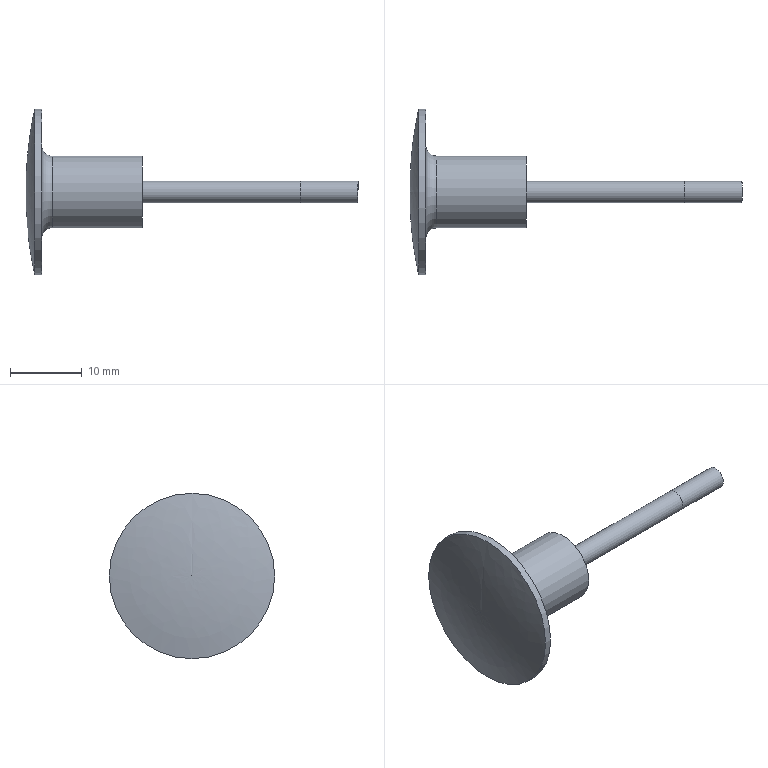Part | STEP file | 1-29.2 | 1 solid | 9 faces | box 46.201 x 23 x 23 mm | volume 2003 mm3 | cylinder 4 | plane 3 | spline 1 | torus 1 | commonest cylinder face diameters 3 x2 10 x1 23 x1
STEP:
#1=CARTESIAN_POINT('',(0.,0.,0.));
#2=DIRECTION('',(0.,0.,1.));
#3=DIRECTION('',(1.,0.,0.));
#4=AXIS2_PLACEMENT_3D('',#1,#2,#3);
#5=CARTESIAN_POINT('',(0.,11.5,0.));
#6=VERTEX_POINT('',#5);
#7=CARTESIAN_POINT('',(-1.,11.5,0.));
#8=VERTEX_POINT('',#7);
#9=CARTESIAN_POINT('',(0.,11.5,0.));
#10=DIRECTION('',(-1.,0.,0.));
#11=VECTOR('',#10,1.);
#12=LINE('',#9,#11);
#13=CARTESIAN_POINT('',(0.,0.,0.));
#14=DIRECTION('',(-1.,0.,0.));
#15=DIRECTION('',(0.,1.,0.));
#16=AXIS2_PLACEMENT_3D('',#13,#14,#15);
#17=CYLINDRICAL_SURFACE('',#16,11.5);
#18=CARTESIAN_POINT('',(6.283,0.));
#19=DIRECTION('',(0.,1.));
#20=VECTOR('',#19,1.);
#21=LINE('',#18,#20);
#22=(GEOMETRIC_REPRESENTATION_CONTEXT(2)PARAMETRIC_REPRESENTATION_CONTEXT()REPRESENTATION_CONTEXT('',''));
#23=DEFINITIONAL_REPRESENTATION('',(#21),#22);
#24=PCURVE('',#17,#23);
#25=CARTESIAN_POINT('',(0.,0.));
#26=DIRECTION('',(0.,1.));
#27=VECTOR('',#26,1.);
#28=LINE('',#25,#27);
#29=(GEOMETRIC_REPRESENTATION_CONTEXT(2)PARAMETRIC_REPRESENTATION_CONTEXT()REPRESENTATION_CONTEXT('',''));
#30=DEFINITIONAL_REPRESENTATION('',(#28),#29);
#31=PCURVE('',#17,#30);
#32=SEAM_CURVE('',#12,(#24,#31),.PCURVE_S1.);
#33=EDGE_CURVE('',#6,#8,#32,.T.);
#34=ORIENTED_EDGE('',*,*,#33,.T.);
#35=CARTESIAN_POINT('',(-1.,0.,11.5));
#36=VERTEX_POINT('',#35);
#37=CARTESIAN_POINT('',(-1.,0.,0.));
#38=DIRECTION('',(1.,0.,0.));
#39=DIRECTION('',(0.,1.,0.));
#40=AXIS2_PLACEMENT_3D('',#37,#38,#39);
#41=CIRCLE('',#40,11.5);
#42=CARTESIAN_POINT('',(6.283,1.));
#43=DIRECTION('',(-1.,0.));
#44=VECTOR('',#43,1.);
#45=LINE('',#42,#44);
#46=(GEOMETRIC_REPRESENTATION_CONTEXT(2)PARAMETRIC_REPRESENTATION_CONTEXT()REPRESENTATION_CONTEXT('',''));
#47=DEFINITIONAL_REPRESENTATION('',(#45),#46);
#48=PCURVE('',#17,#47);
#49=CARTESIAN_POINT('',(-1.,0.,11.5));
#50=CARTESIAN_POINT('',(-1.,-11.5,11.5));
#51=CARTESIAN_POINT('',(-1.,-11.5,0.));
#52=CARTESIAN_POINT('',(-1.,-11.5,-11.5));
#53=CARTESIAN_POINT('',(-1.,0.,-11.5));
#54=CARTESIAN_POINT('',(-1.,11.5,-11.5));
#55=CARTESIAN_POINT('',(-1.,11.5,0.));
#56=CARTESIAN_POINT('',(-1.,11.5,11.5));
#57=CARTESIAN_POINT('',(-1.,0.,11.5));
#58=CARTESIAN_POINT('',(-2.243,0.,5.817));
#59=CARTESIAN_POINT('',(-2.243,-5.817,5.817));
#60=CARTESIAN_POINT('',(-2.243,-5.817,0.));
#61=CARTESIAN_POINT('',(-2.243,-5.817,-5.817));
#62=CARTESIAN_POINT('',(-2.243,0.,-5.817));
#63=CARTESIAN_POINT('',(-2.243,5.817,-5.817));
#64=CARTESIAN_POINT('',(-2.243,5.817,0.));
#65=CARTESIAN_POINT('',(-2.243,5.817,5.817));
#66=CARTESIAN_POINT('',(-2.243,0.,5.817));
#67=CARTESIAN_POINT('',(-2.2,0.,0.));
#68=CARTESIAN_POINT('',(-2.2,0.,0.));
#69=CARTESIAN_POINT('',(-2.2,0.,0.));
#70=CARTESIAN_POINT('',(-2.2,0.,0.));
#71=CARTESIAN_POINT('',(-2.2,0.,0.));
#72=CARTESIAN_POINT('',(-2.2,0.,0.));
#73=CARTESIAN_POINT('',(-2.2,0.,0.));
#74=CARTESIAN_POINT('',(-2.2,0.,0.));
#75=CARTESIAN_POINT('',(-2.2,0.,0.));
#76=(BOUNDED_SURFACE()B_SPLINE_SURFACE(2,2,((#49,#50,#51,#52,#53,#54,#55,#56,#57),(#58,#59,#60,#61,#62,#63,#64,#65,#66),(#67,#68,#69,#70,#71,#72,#73,#74,#75)),.UNSPECIFIED.,.F.,.T.,.F.)B_SPLINE_SURFACE_WITH_KNOTS((3,3),(1,2,2,2,2,2,1),(0.,1.),(-0.25,0.,0.25,0.5,0.75,1.,1.25),.UNSPECIFIED.)GEOMETRIC_REPRESENTATION_ITEM()RATIONAL_B_SPLINE_SURFACE(((1.,0.7071,1.,0.7071,1.,0.7071,1.,0.7071,1.),(0.9938,0.7027,0.9938,0.7027,0.9938,0.7027,0.9938,0.7027,0.9938),(1.,0.7071,1.,0.7071,1.,0.7071,1.,0.7071,1.)))REPRESENTATION_ITEM('')SURFACE());
#77=CARTESIAN_POINT('',(0.,0.75));
#78=CARTESIAN_POINT('',(0.,0.7542));
#79=CARTESIAN_POINT('',(0.,0.7625));
#80=CARTESIAN_POINT('',(0.,0.7746));
#81=CARTESIAN_POINT('',(0.,0.7864));
#82=CARTESIAN_POINT('',(0.,0.798));
#83=CARTESIAN_POINT('',(0.,0.8094));
#84=CARTESIAN_POINT('',(0.,0.8206));
#85=CARTESIAN_POINT('',(0.,0.8316));
#86=CARTESIAN_POINT('',(0.,0.8426));
#87=CARTESIAN_POINT('',(0.,0.8534));
#88=CARTESIAN_POINT('',(0.,0.8642));
#89=CARTESIAN_POINT('',(0.,0.875));
#90=CARTESIAN_POINT('',(0.,0.8858));
#91=CARTESIAN_POINT('',(0.,0.8966));
#92=CARTESIAN_POINT('',(0.,0.9074));
#93=CARTESIAN_POINT('',(0.,0.9184));
#94=CARTESIAN_POINT('',(0.,0.9294));
#95=CARTESIAN_POINT('',(0.,0.9406));
#96=CARTESIAN_POINT('',(0.,0.952));
#97=CARTESIAN_POINT('',(0.,0.9636));
#98=CARTESIAN_POINT('',(0.,0.9754));
#99=CARTESIAN_POINT('',(0.,0.9875));
#100=CARTESIAN_POINT('',(0.,0.9958));
#101=CARTESIAN_POINT('',(0.,1.));
#102=B_SPLINE_CURVE_WITH_KNOTS('',3,(#77,#78,#79,#80,#81,#82,#83,#84,#85,#86,#87,#88,#89,#90,#91,#92,#93,#94,#95,#96,#97,#98,#99,#100,#101),.UNSPECIFIED.,.F.,.F.,(4,1,1,1,1,1,1,1,1,1,1,1,1,1,1,1,1,1,1,1,1,1,4),(0.,0.0714,0.1428,0.2142,0.2856,0.357,0.4284,0.4998,0.5712,0.6426,0.714,0.7854,0.8568,0.9282,0.9996,1.071,1.142,1.214,1.285,1.357,1.428,1.499,1.571),.QUASI_UNIFORM_KNOTS.);
#103=(GEOMETRIC_REPRESENTATION_CONTEXT(2)PARAMETRIC_REPRESENTATION_CONTEXT()REPRESENTATION_CONTEXT('',''));
#104=DEFINITIONAL_REPRESENTATION('',(#102),#103);
#105=PCURVE('',#76,#104);
#106=SURFACE_CURVE('',#41,(#48,#105),.PCURVE_S1.);
#107=EDGE_CURVE('',#8,#36,#106,.T.);
#108=ORIENTED_EDGE('',*,*,#107,.T.);
#109=CARTESIAN_POINT('',(-1.,0.,0.));
#110=DIRECTION('',(1.,0.,0.));
#111=DIRECTION('',(0.,0.,1.));
#112=AXIS2_PLACEMENT_3D('',#109,#110,#111);
#113=CIRCLE('',#112,11.5);
#114=CARTESIAN_POINT('',(4.712,1.));
#115=DIRECTION('',(-1.,0.));
#116=VECTOR('',#115,1.);
#117=LINE('',#114,#116);
#118=(GEOMETRIC_REPRESENTATION_CONTEXT(2)PARAMETRIC_REPRESENTATION_CONTEXT()REPRESENTATION_CONTEXT('',''));
#119=DEFINITIONAL_REPRESENTATION('',(#117),#118);
#120=PCURVE('',#17,#119);
#121=CARTESIAN_POINT('',(0.,0.));
#122=CARTESIAN_POINT('',(0.,0.0126));
#123=CARTESIAN_POINT('',(0.,0.03676));
#124=CARTESIAN_POINT('',(0.,0.07076));
#125=CARTESIAN_POINT('',(0.,0.1035));
#126=CARTESIAN_POINT('',(0.,0.1357));
#127=CARTESIAN_POINT('',(0.,0.1682));
#128=CARTESIAN_POINT('',(0.,0.2017));
#129=CARTESIAN_POINT('',(0.,0.2371));
#130=CARTESIAN_POINT('',(0.,0.2752));
#131=CARTESIAN_POINT('',(0.,0.3096));
#132=CARTESIAN_POINT('',(0.,0.3427));
#133=CARTESIAN_POINT('',(0.,0.375));
#134=CARTESIAN_POINT('',(0.,0.4073));
#135=CARTESIAN_POINT('',(0.,0.4404));
#136=CARTESIAN_POINT('',(0.,0.4748));
#137=CARTESIAN_POINT('',(0.,0.5129));
#138=CARTESIAN_POINT('',(0.,0.5483));
#139=CARTESIAN_POINT('',(0.,0.5818));
#140=CARTESIAN_POINT('',(0.,0.6143));
#141=CARTESIAN_POINT('',(0.,0.6465));
#142=CARTESIAN_POINT('',(0.,0.6792));
#143=CARTESIAN_POINT('',(0.,0.7132));
#144=CARTESIAN_POINT('',(0.,0.7374));
#145=CARTESIAN_POINT('',(0.,0.75));
#146=B_SPLINE_CURVE_WITH_KNOTS('',3,(#121,#122,#123,#124,#125,#126,#127,#128,#129,#130,#131,#132,#133,#134,#135,#136,#137,#138,#139,#140,#141,#142,#143,#144,#145),.UNSPECIFIED.,.F.,.F.,(4,1,1,1,1,1,1,1,1,1,1,1,1,1,1,1,1,1,1,1,1,1,4),(0.,0.2142,0.4284,0.6426,0.8568,1.071,1.285,1.499,1.714,1.928,2.142,2.356,2.57,2.785,2.999,3.213,3.427,3.641,3.856,4.07,4.284,4.498,4.712),.QUASI_UNIFORM_KNOTS.);
#147=(GEOMETRIC_REPRESENTATION_CONTEXT(2)PARAMETRIC_REPRESENTATION_CONTEXT()REPRESENTATION_CONTEXT('',''));
#148=DEFINITIONAL_REPRESENTATION('',(#146),#147);
#149=PCURVE('',#76,#148);
#150=SURFACE_CURVE('',#113,(#120,#149),.PCURVE_S1.);
#151=EDGE_CURVE('',#36,#8,#150,.T.);
#152=ORIENTED_EDGE('',*,*,#151,.T.);
#153=ORIENTED_EDGE('',*,*,#33,.F.);
#154=CARTESIAN_POINT('',(0.,0.,0.));
#155=DIRECTION('',(1.,0.,0.));
#156=DIRECTION('',(0.,1.,0.));
#157=AXIS2_PLACEMENT_3D('',#154,#155,#156);
#158=CIRCLE('',#157,11.5);
#159=CARTESIAN_POINT('',(6.283,0.));
#160=DIRECTION('',(-1.,0.));
#161=VECTOR('',#160,1.);
#162=LINE('',#159,#161);
#163=(GEOMETRIC_REPRESENTATION_CONTEXT(2)PARAMETRIC_REPRESENTATION_CONTEXT()REPRESENTATION_CONTEXT('',''));
#164=DEFINITIONAL_REPRESENTATION('',(#162),#163);
#165=PCURVE('',#17,#164);
#166=CARTESIAN_POINT('',(0.,-3.081,0.));
#167=DIRECTION('',(1.,0.,0.));
#168=DIRECTION('',(0.,0.,-1.));
#169=AXIS2_PLACEMENT_3D('',#166,#167,#168);
#170=PLANE('',#169);
#171=CARTESIAN_POINT('',(0.,3.081));
#172=DIRECTION('',(0.,1.));
#173=AXIS2_PLACEMENT_2D('',#171,#172);
#174=CIRCLE('',#173,11.5);
#175=(GEOMETRIC_REPRESENTATION_CONTEXT(2)PARAMETRIC_REPRESENTATION_CONTEXT()REPRESENTATION_CONTEXT('',''));
#176=DEFINITIONAL_REPRESENTATION('',(#174),#175);
#177=PCURVE('',#170,#176);
#178=SURFACE_CURVE('',#158,(#165,#177),.PCURVE_S1.);
#179=EDGE_CURVE('',#6,#6,#178,.T.);
#180=ORIENTED_EDGE('',*,*,#179,.F.);
#181=EDGE_LOOP('',(#34,#108,#152,#153,#180));
#182=FACE_BOUND('',#181,.T.);
#183=ADVANCED_FACE('',(#182),#17,.T.);
#184=CARTESIAN_POINT('',(-2.2,0.,0.));
#185=VERTEX_POINT('',#184);
#186=CARTESIAN_POINT('',(49.799,0.,0.3867));
#187=DIRECTION('',(0.,-1.,0.));
#188=DIRECTION('',(-0.9769,0.,0.2137));
#189=AXIS2_PLACEMENT_3D('',#186,#187,#188);
#190=CIRCLE('',#189,52.);
#191=CARTESIAN_POINT('',(0.,0.));
#192=CARTESIAN_POINT('',(0.01518,0.));
#193=CARTESIAN_POINT('',(0.04554,0.));
#194=CARTESIAN_POINT('',(0.09105,0.));
#195=CARTESIAN_POINT('',(0.1365,0.));
#196=CARTESIAN_POINT('',(0.182,0.));
#197=CARTESIAN_POINT('',(0.2275,0.));
#198=CARTESIAN_POINT('',(0.2729,0.));
#199=CARTESIAN_POINT('',(0.3183,0.));
#200=CARTESIAN_POINT('',(0.3638,0.));
#201=CARTESIAN_POINT('',(0.4092,0.));
#202=CARTESIAN_POINT('',(0.4546,0.));
#203=CARTESIAN_POINT('',(0.5,0.));
#204=CARTESIAN_POINT('',(0.5454,0.));
#205=CARTESIAN_POINT('',(0.5908,0.));
#206=CARTESIAN_POINT('',(0.6362,0.));
#207=CARTESIAN_POINT('',(0.6817,0.));
#208=CARTESIAN_POINT('',(0.7271,0.));
#209=CARTESIAN_POINT('',(0.7725,0.));
#210=CARTESIAN_POINT('',(0.818,0.));
#211=CARTESIAN_POINT('',(0.8635,0.));
#212=CARTESIAN_POINT('',(0.9089,0.));
#213=CARTESIAN_POINT('',(0.9545,0.));
#214=CARTESIAN_POINT('',(0.9848,0.));
#215=CARTESIAN_POINT('',(1.,0.));
#216=B_SPLINE_CURVE_WITH_KNOTS('',3,(#191,#192,#193,#194,#195,#196,#197,#198,#199,#200,#201,#202,#203,#204,#205,#206,#207,#208,#209,#210,#211,#212,#213,#214,#215),.UNSPECIFIED.,.F.,.F.,(4,1,1,1,1,1,1,1,1,1,1,1,1,1,1,1,1,1,1,1,1,1,4),(0.,0.01013,0.02026,0.03038,0.04051,0.05064,0.06077,0.0709,0.08102,0.09115,0.1013,0.1114,0.1215,0.1317,0.1418,0.1519,0.162,0.1722,0.1823,0.1924,0.2026,0.2127,0.2228),.QUASI_UNIFORM_KNOTS.);
#217=(GEOMETRIC_REPRESENTATION_CONTEXT(2)PARAMETRIC_REPRESENTATION_CONTEXT()REPRESENTATION_CONTEXT('',''));
#218=DEFINITIONAL_REPRESENTATION('',(#216),#217);
#219=PCURVE('',#76,#218);
#220=CARTESIAN_POINT('',(0.,1.));
#221=CARTESIAN_POINT('',(0.01518,1.));
#222=CARTESIAN_POINT('',(0.04554,1.));
#223=CARTESIAN_POINT('',(0.09105,1.));
#224=CARTESIAN_POINT('',(0.1365,1.));
#225=CARTESIAN_POINT('',(0.182,1.));
#226=CARTESIAN_POINT('',(0.2275,1.));
#227=CARTESIAN_POINT('',(0.2729,1.));
#228=CARTESIAN_POINT('',(0.3183,1.));
#229=CARTESIAN_POINT('',(0.3638,1.));
#230=CARTESIAN_POINT('',(0.4092,1.));
#231=CARTESIAN_POINT('',(0.4546,1.));
#232=CARTESIAN_POINT('',(0.5,1.));
#233=CARTESIAN_POINT('',(0.5454,1.));
#234=CARTESIAN_POINT('',(0.5908,1.));
#235=CARTESIAN_POINT('',(0.6362,1.));
#236=CARTESIAN_POINT('',(0.6817,1.));
#237=CARTESIAN_POINT('',(0.7271,1.));
#238=CARTESIAN_POINT('',(0.7725,1.));
#239=CARTESIAN_POINT('',(0.818,1.));
#240=CARTESIAN_POINT('',(0.8635,1.));
#241=CARTESIAN_POINT('',(0.9089,1.));
#242=CARTESIAN_POINT('',(0.9545,1.));
#243=CARTESIAN_POINT('',(0.9848,1.));
#244=CARTESIAN_POINT('',(1.,1.));
#245=B_SPLINE_CURVE_WITH_KNOTS('',3,(#220,#221,#222,#223,#224,#225,#226,#227,#228,#229,#230,#231,#232,#233,#234,#235,#236,#237,#238,#239,#240,#241,#242,#243,#244),.UNSPECIFIED.,.F.,.F.,(4,1,1,1,1,1,1,1,1,1,1,1,1,1,1,1,1,1,1,1,1,1,4),(0.,0.01013,0.02026,0.03038,0.04051,0.05064,0.06077,0.0709,0.08102,0.09115,0.1013,0.1114,0.1215,0.1317,0.1418,0.1519,0.162,0.1722,0.1823,0.1924,0.2026,0.2127,0.2228),.QUASI_UNIFORM_KNOTS.);
#246=(GEOMETRIC_REPRESENTATION_CONTEXT(2)PARAMETRIC_REPRESENTATION_CONTEXT()REPRESENTATION_CONTEXT('',''));
#247=DEFINITIONAL_REPRESENTATION('',(#245),#246);
#248=PCURVE('',#76,#247);
#249=SEAM_CURVE('',#190,(#219,#248),.PCURVE_S1.);
#250=EDGE_CURVE('',#36,#185,#249,.T.);
#251=ORIENTED_EDGE('',*,*,#250,.T.);
#252=ORIENTED_EDGE('',*,*,#250,.F.);
#253=ORIENTED_EDGE('',*,*,#107,.F.);
#254=ORIENTED_EDGE('',*,*,#151,.F.);
#255=EDGE_LOOP('',(#251,#252,#253,#254));
#256=FACE_BOUND('',#255,.T.);
#257=ADVANCED_FACE('',(#256),#76,.T.);
#258=CARTESIAN_POINT('',(14.,5.,0.));
#259=VERTEX_POINT('',#258);
#260=CARTESIAN_POINT('',(14.,0.,0.));
#261=DIRECTION('',(1.,0.,0.));
#262=DIRECTION('',(0.,1.,0.));
#263=AXIS2_PLACEMENT_3D('',#260,#261,#262);
#264=CIRCLE('',#263,5.);
#265=CARTESIAN_POINT('',(0.,0.,0.));
#266=DIRECTION('',(1.,0.,0.));
#267=DIRECTION('',(0.,1.,0.));
#268=AXIS2_PLACEMENT_3D('',#265,#266,#267);
#269=CYLINDRICAL_SURFACE('',#268,5.);
#270=CARTESIAN_POINT('',(0.,14.));
#271=DIRECTION('',(1.,0.));
#272=VECTOR('',#271,1.);
#273=LINE('',#270,#272);
#274=(GEOMETRIC_REPRESENTATION_CONTEXT(2)PARAMETRIC_REPRESENTATION_CONTEXT()REPRESENTATION_CONTEXT('',''));
#275=DEFINITIONAL_REPRESENTATION('',(#273),#274);
#276=PCURVE('',#269,#275);
#277=CARTESIAN_POINT('',(14.,-1.34,0.));
#278=DIRECTION('',(1.,0.,0.));
#279=DIRECTION('',(0.,0.,-1.));
#280=AXIS2_PLACEMENT_3D('',#277,#278,#279);
#281=PLANE('',#280);
#282=CARTESIAN_POINT('',(0.,1.34));
#283=DIRECTION('',(0.,1.));
#284=AXIS2_PLACEMENT_2D('',#282,#283);
#285=CIRCLE('',#284,5.);
#286=(GEOMETRIC_REPRESENTATION_CONTEXT(2)PARAMETRIC_REPRESENTATION_CONTEXT()REPRESENTATION_CONTEXT('',''));
#287=DEFINITIONAL_REPRESENTATION('',(#285),#286);
#288=PCURVE('',#281,#287);
#289=SURFACE_CURVE('',#264,(#276,#288),.PCURVE_S1.);
#290=EDGE_CURVE('',#259,#259,#289,.T.);
#291=ORIENTED_EDGE('',*,*,#290,.F.);
#292=CARTESIAN_POINT('',(1.5,5.,0.));
#293=VERTEX_POINT('',#292);
#294=CARTESIAN_POINT('',(1.5,5.,0.));
#295=DIRECTION('',(1.,0.,0.));
#296=VECTOR('',#295,1.);
#297=LINE('',#294,#296);
#298=CARTESIAN_POINT('',(0.,1.5));
#299=DIRECTION('',(0.,1.));
#300=VECTOR('',#299,1.);
#301=LINE('',#298,#300);
#302=(GEOMETRIC_REPRESENTATION_CONTEXT(2)PARAMETRIC_REPRESENTATION_CONTEXT()REPRESENTATION_CONTEXT('',''));
#303=DEFINITIONAL_REPRESENTATION('',(#301),#302);
#304=PCURVE('',#269,#303);
#305=CARTESIAN_POINT('',(6.283,1.5));
#306=DIRECTION('',(0.,1.));
#307=VECTOR('',#306,1.);
#308=LINE('',#305,#307);
#309=(GEOMETRIC_REPRESENTATION_CONTEXT(2)PARAMETRIC_REPRESENTATION_CONTEXT()REPRESENTATION_CONTEXT('',''));
#310=DEFINITIONAL_REPRESENTATION('',(#308),#309);
#311=PCURVE('',#269,#310);
#312=SEAM_CURVE('',#297,(#304,#311),.PCURVE_S1.);
#313=EDGE_CURVE('',#293,#259,#312,.T.);
#314=ORIENTED_EDGE('',*,*,#313,.F.);
#315=CARTESIAN_POINT('',(1.5,0.,0.));
#316=DIRECTION('',(-1.,0.,0.));
#317=DIRECTION('',(0.,1.,0.));
#318=AXIS2_PLACEMENT_3D('',#315,#316,#317);
#319=CIRCLE('',#318,5.);
#320=CARTESIAN_POINT('',(6.283,1.5));
#321=DIRECTION('',(-1.,0.));
#322=VECTOR('',#321,1.);
#323=LINE('',#320,#322);
#324=(GEOMETRIC_REPRESENTATION_CONTEXT(2)PARAMETRIC_REPRESENTATION_CONTEXT()REPRESENTATION_CONTEXT('',''));
#325=DEFINITIONAL_REPRESENTATION('',(#323),#324);
#326=PCURVE('',#269,#325);
#327=CARTESIAN_POINT('',(1.5,0.,0.));
#328=DIRECTION('',(1.,0.,0.));
#329=DIRECTION('',(0.,1.,0.));
#330=AXIS2_PLACEMENT_3D('',#327,#328,#329);
#331=TOROIDAL_SURFACE('',#330,6.5,1.5);
#332=CARTESIAN_POINT('',(6.283,3.142));
#333=DIRECTION('',(-1.,0.));
#334=VECTOR('',#333,1.);
#335=LINE('',#332,#334);
#336=(GEOMETRIC_REPRESENTATION_CONTEXT(2)PARAMETRIC_REPRESENTATION_CONTEXT()REPRESENTATION_CONTEXT('',''));
#337=DEFINITIONAL_REPRESENTATION('',(#335),#336);
#338=PCURVE('',#331,#337);
#339=SURFACE_CURVE('',#319,(#326,#338),.PCURVE_S1.);
#340=EDGE_CURVE('',#293,#293,#339,.T.);
#341=ORIENTED_EDGE('',*,*,#340,.F.);
#342=ORIENTED_EDGE('',*,*,#313,.T.);
#343=EDGE_LOOP('',(#291,#314,#341,#342));
#344=FACE_BOUND('',#343,.T.);
#345=ADVANCED_FACE('',(#344),#269,.T.);
#346=ORIENTED_EDGE('',*,*,#179,.T.);
#347=EDGE_LOOP('',(#346));
#348=FACE_BOUND('',#347,.T.);
#349=CARTESIAN_POINT('',(0.,6.5,0.));
#350=VERTEX_POINT('',#349);
#351=CARTESIAN_POINT('',(0.,0.,0.));
#352=DIRECTION('',(-1.,0.,0.));
#353=DIRECTION('',(0.,1.,0.));
#354=AXIS2_PLACEMENT_3D('',#351,#352,#353);
#355=CIRCLE('',#354,6.5);
#356=CARTESIAN_POINT('',(0.,9.581));
#357=CARTESIAN_POINT('',(11.258,9.581));
#358=CARTESIAN_POINT('',(5.629,-0.1686));
#359=CARTESIAN_POINT('',(0.,-9.919));
#360=CARTESIAN_POINT('',(-5.629,-0.1686));
#361=CARTESIAN_POINT('',(-11.258,9.581));
#362=CARTESIAN_POINT('',(0.,9.581));
#363=(BOUNDED_CURVE()B_SPLINE_CURVE(2,(#356,#357,#358,#359,#360,#361,#362),.UNSPECIFIED.,.T.,.F.)B_SPLINE_CURVE_WITH_KNOTS((1,2,2,2,2,1),(-2.094,0.,2.094,4.189,6.283,8.378),.UNSPECIFIED.)CURVE()GEOMETRIC_REPRESENTATION_ITEM()RATIONAL_B_SPLINE_CURVE((1.,0.5,1.,0.5,1.,0.5,1.))REPRESENTATION_ITEM(''));
#364=(GEOMETRIC_REPRESENTATION_CONTEXT(2)PARAMETRIC_REPRESENTATION_CONTEXT()REPRESENTATION_CONTEXT('',''));
#365=DEFINITIONAL_REPRESENTATION('',(#363),#364);
#366=PCURVE('',#170,#365);
#367=CARTESIAN_POINT('',(6.283,4.712));
#368=DIRECTION('',(-1.,0.));
#369=VECTOR('',#368,1.);
#370=LINE('',#367,#369);
#371=(GEOMETRIC_REPRESENTATION_CONTEXT(2)PARAMETRIC_REPRESENTATION_CONTEXT()REPRESENTATION_CONTEXT('',''));
#372=DEFINITIONAL_REPRESENTATION('',(#370),#371);
#373=PCURVE('',#331,#372);
#374=SURFACE_CURVE('',#355,(#366,#373),.PCURVE_S1.);
#375=EDGE_CURVE('',#350,#350,#374,.T.);
#376=ORIENTED_EDGE('',*,*,#375,.T.);
#377=EDGE_LOOP('',(#376));
#378=FACE_BOUND('',#377,.T.);
#379=ADVANCED_FACE('',(#348,#378),#170,.T.);
#380=CARTESIAN_POINT('',(1.5,6.5,0.));
#381=DIRECTION('',(0.,0.,-1.));
#382=DIRECTION('',(0.,-1.,0.));
#383=AXIS2_PLACEMENT_3D('',#380,#381,#382);
#384=CIRCLE('',#383,1.5);
#385=CARTESIAN_POINT('',(0.,3.142));
#386=DIRECTION('',(0.,1.));
#387=VECTOR('',#386,1.);
#388=LINE('',#385,#387);
#389=(GEOMETRIC_REPRESENTATION_CONTEXT(2)PARAMETRIC_REPRESENTATION_CONTEXT()REPRESENTATION_CONTEXT('',''));
#390=DEFINITIONAL_REPRESENTATION('',(#388),#389);
#391=PCURVE('',#331,#390);
#392=CARTESIAN_POINT('',(6.283,3.142));
#393=DIRECTION('',(0.,1.));
#394=VECTOR('',#393,1.);
#395=LINE('',#392,#394);
#396=(GEOMETRIC_REPRESENTATION_CONTEXT(2)PARAMETRIC_REPRESENTATION_CONTEXT()REPRESENTATION_CONTEXT('',''));
#397=DEFINITIONAL_REPRESENTATION('',(#395),#396);
#398=PCURVE('',#331,#397);
#399=SEAM_CURVE('',#384,(#391,#398),.PCURVE_S1.);
#400=EDGE_CURVE('',#293,#350,#399,.T.);
#401=ORIENTED_EDGE('',*,*,#400,.F.);
#402=ORIENTED_EDGE('',*,*,#340,.F.);
#403=ORIENTED_EDGE('',*,*,#400,.T.);
#404=ORIENTED_EDGE('',*,*,#375,.T.);
#405=EDGE_LOOP('',(#401,#402,#403,#404));
#406=FACE_BOUND('',#405,.F.);
#407=ADVANCED_FACE('',(#406),#331,.F.);
#408=ORIENTED_EDGE('',*,*,#290,.T.);
#409=EDGE_LOOP('',(#408));
#410=FACE_BOUND('',#409,.T.);
#411=CARTESIAN_POINT('',(14.,1.5,0.));
#412=VERTEX_POINT('',#411);
#413=CARTESIAN_POINT('',(14.,0.,0.));
#414=DIRECTION('',(1.,0.,0.));
#415=DIRECTION('',(0.,1.,0.));
#416=AXIS2_PLACEMENT_3D('',#413,#414,#415);
#417=CIRCLE('',#416,1.5);
#418=CARTESIAN_POINT('',(0.,1.34));
#419=DIRECTION('',(0.,1.));
#420=AXIS2_PLACEMENT_2D('',#418,#419);
#421=CIRCLE('',#420,1.5);
#422=(GEOMETRIC_REPRESENTATION_CONTEXT(2)PARAMETRIC_REPRESENTATION_CONTEXT()REPRESENTATION_CONTEXT('',''));
#423=DEFINITIONAL_REPRESENTATION('',(#421),#422);
#424=PCURVE('',#281,#423);
#425=CARTESIAN_POINT('',(14.,0.,0.));
#426=DIRECTION('',(1.,0.,0.));
#427=DIRECTION('',(0.,1.,0.));
#428=AXIS2_PLACEMENT_3D('',#425,#426,#427);
#429=CYLINDRICAL_SURFACE('',#428,1.5);
#430=CARTESIAN_POINT('',(0.,0.));
#431=DIRECTION('',(1.,0.));
#432=VECTOR('',#431,1.);
#433=LINE('',#430,#432);
#434=(GEOMETRIC_REPRESENTATION_CONTEXT(2)PARAMETRIC_REPRESENTATION_CONTEXT()REPRESENTATION_CONTEXT('',''));
#435=DEFINITIONAL_REPRESENTATION('',(#433),#434);
#436=PCURVE('',#429,#435);
#437=SURFACE_CURVE('',#417,(#424,#436),.PCURVE_S1.);
#438=EDGE_CURVE('',#412,#412,#437,.T.);
#439=ORIENTED_EDGE('',*,*,#438,.F.);
#440=EDGE_LOOP('',(#439));
#441=FACE_BOUND('',#440,.T.);
#442=ADVANCED_FACE('',(#410,#441),#281,.T.);
#443=CARTESIAN_POINT('',(44.,1.5,0.));
#444=VERTEX_POINT('',#443);
#445=CARTESIAN_POINT('',(44.,0.,0.));
#446=DIRECTION('',(1.,0.,0.));
#447=DIRECTION('',(0.,1.,0.));
#448=AXIS2_PLACEMENT_3D('',#445,#446,#447);
#449=CIRCLE('',#448,1.5);
#450=CARTESIAN_POINT('',(44.,-0.4019,0.));
#451=DIRECTION('',(1.,0.,0.));
#452=DIRECTION('',(0.,1.,0.));
#453=AXIS2_PLACEMENT_3D('',#450,#451,#452);
#454=PLANE('',#453);
#455=CARTESIAN_POINT('',(0.4019,0.));
#456=DIRECTION('',(1.,0.));
#457=AXIS2_PLACEMENT_2D('',#455,#456);
#458=CIRCLE('',#457,1.5);
#459=(GEOMETRIC_REPRESENTATION_CONTEXT(2)PARAMETRIC_REPRESENTATION_CONTEXT()REPRESENTATION_CONTEXT('',''));
#460=DEFINITIONAL_REPRESENTATION('',(#458),#459);
#461=PCURVE('',#454,#460);
#462=CARTESIAN_POINT('',(36.,0.,0.));
#463=DIRECTION('',(1.,0.,0.));
#464=DIRECTION('',(0.,1.,0.));
#465=AXIS2_PLACEMENT_3D('',#462,#463,#464);
#466=CYLINDRICAL_SURFACE('',#465,1.5);
#467=CARTESIAN_POINT('',(0.,8.));
#468=DIRECTION('',(1.,0.));
#469=VECTOR('',#468,1.);
#470=LINE('',#467,#469);
#471=(GEOMETRIC_REPRESENTATION_CONTEXT(2)PARAMETRIC_REPRESENTATION_CONTEXT()REPRESENTATION_CONTEXT('',''));
#472=DEFINITIONAL_REPRESENTATION('',(#470),#471);
#473=PCURVE('',#466,#472);
#474=SURFACE_CURVE('',#449,(#461,#473),.PCURVE_S1.);
#475=EDGE_CURVE('',#444,#444,#474,.T.);
#476=ORIENTED_EDGE('',*,*,#475,.T.);
#477=EDGE_LOOP('',(#476));
#478=FACE_BOUND('',#477,.T.);
#479=ADVANCED_FACE('',(#478),#454,.T.);
#480=ORIENTED_EDGE('',*,*,#438,.T.);
#481=CARTESIAN_POINT('',(36.,1.5,0.));
#482=VERTEX_POINT('',#481);
#483=CARTESIAN_POINT('',(14.,1.5,0.));
#484=DIRECTION('',(1.,0.,0.));
#485=VECTOR('',#484,1.);
#486=LINE('',#483,#485);
#487=CARTESIAN_POINT('',(6.283,0.));
#488=DIRECTION('',(0.,1.));
#489=VECTOR('',#488,1.);
#490=LINE('',#487,#489);
#491=(GEOMETRIC_REPRESENTATION_CONTEXT(2)PARAMETRIC_REPRESENTATION_CONTEXT()REPRESENTATION_CONTEXT('',''));
#492=DEFINITIONAL_REPRESENTATION('',(#490),#491);
#493=PCURVE('',#429,#492);
#494=CARTESIAN_POINT('',(0.,0.));
#495=DIRECTION('',(0.,1.));
#496=VECTOR('',#495,1.);
#497=LINE('',#494,#496);
#498=(GEOMETRIC_REPRESENTATION_CONTEXT(2)PARAMETRIC_REPRESENTATION_CONTEXT()REPRESENTATION_CONTEXT('',''));
#499=DEFINITIONAL_REPRESENTATION('',(#497),#498);
#500=PCURVE('',#429,#499);
#501=SEAM_CURVE('',#486,(#493,#500),.PCURVE_S1.);
#502=EDGE_CURVE('',#412,#482,#501,.T.);
#503=ORIENTED_EDGE('',*,*,#502,.T.);
#504=CARTESIAN_POINT('',(36.,0.,0.));
#505=DIRECTION('',(1.,0.,0.));
#506=DIRECTION('',(0.,1.,0.));
#507=AXIS2_PLACEMENT_3D('',#504,#505,#506);
#508=CIRCLE('',#507,1.5);
#509=CARTESIAN_POINT('',(0.,22.));
#510=DIRECTION('',(1.,0.));
#511=VECTOR('',#510,1.);
#512=LINE('',#509,#511);
#513=(GEOMETRIC_REPRESENTATION_CONTEXT(2)PARAMETRIC_REPRESENTATION_CONTEXT()REPRESENTATION_CONTEXT('',''));
#514=DEFINITIONAL_REPRESENTATION('',(#512),#513);
#515=PCURVE('',#429,#514);
#516=CARTESIAN_POINT('',(0.,0.));
#517=DIRECTION('',(1.,0.));
#518=VECTOR('',#517,1.);
#519=LINE('',#516,#518);
#520=(GEOMETRIC_REPRESENTATION_CONTEXT(2)PARAMETRIC_REPRESENTATION_CONTEXT()REPRESENTATION_CONTEXT('',''));
#521=DEFINITIONAL_REPRESENTATION('',(#519),#520);
#522=PCURVE('',#466,#521);
#523=SURFACE_CURVE('',#508,(#515,#522),.PCURVE_S1.);
#524=EDGE_CURVE('',#482,#482,#523,.T.);
#525=ORIENTED_EDGE('',*,*,#524,.F.);
#526=ORIENTED_EDGE('',*,*,#502,.F.);
#527=EDGE_LOOP('',(#480,#503,#525,#526));
#528=FACE_BOUND('',#527,.T.);
#529=ADVANCED_FACE('',(#528),#429,.T.);
#530=ORIENTED_EDGE('',*,*,#475,.F.);
#531=CARTESIAN_POINT('',(36.,1.5,0.));
#532=DIRECTION('',(1.,0.,0.));
#533=VECTOR('',#532,1.);
#534=LINE('',#531,#533);
#535=CARTESIAN_POINT('',(0.,0.));
#536=DIRECTION('',(0.,1.));
#537=VECTOR('',#536,1.);
#538=LINE('',#535,#537);
#539=(GEOMETRIC_REPRESENTATION_CONTEXT(2)PARAMETRIC_REPRESENTATION_CONTEXT()REPRESENTATION_CONTEXT('',''));
#540=DEFINITIONAL_REPRESENTATION('',(#538),#539);
#541=PCURVE('',#466,#540);
#542=CARTESIAN_POINT('',(6.283,0.));
#543=DIRECTION('',(0.,1.));
#544=VECTOR('',#543,1.);
#545=LINE('',#542,#544);
#546=(GEOMETRIC_REPRESENTATION_CONTEXT(2)PARAMETRIC_REPRESENTATION_CONTEXT()REPRESENTATION_CONTEXT('',''));
#547=DEFINITIONAL_REPRESENTATION('',(#545),#546);
#548=PCURVE('',#466,#547);
#549=SEAM_CURVE('',#534,(#541,#548),.PCURVE_S1.);
#550=EDGE_CURVE('',#482,#444,#549,.T.);
#551=ORIENTED_EDGE('',*,*,#550,.F.);
#552=ORIENTED_EDGE('',*,*,#524,.T.);
#553=ORIENTED_EDGE('',*,*,#550,.T.);
#554=EDGE_LOOP('',(#530,#551,#552,#553));
#555=FACE_BOUND('',#554,.T.);
#556=ADVANCED_FACE('',(#555),#466,.T.);
#557=CLOSED_SHELL('',(#183,#257,#345,#379,#407,#442,#479,#529,#556));
#558=MANIFOLD_SOLID_BREP('',#557);
#559=(LENGTH_UNIT()NAMED_UNIT(*)SI_UNIT(.MILLI.,.METRE.));
#560=UNCERTAINTY_MEASURE_WITH_UNIT(LENGTH_MEASURE(0.0000001),#559,'','');
#561=(NAMED_UNIT(*)PLANE_ANGLE_UNIT()SI_UNIT($,.RADIAN.));
#562=(NAMED_UNIT(*)SI_UNIT($,.STERADIAN.)SOLID_ANGLE_UNIT());
#563=(GEOMETRIC_REPRESENTATION_CONTEXT(3)GLOBAL_UNCERTAINTY_ASSIGNED_CONTEXT((#560))GLOBAL_UNIT_ASSIGNED_CONTEXT((#559,#561,#562))REPRESENTATION_CONTEXT('',''));
#564=ADVANCED_BREP_SHAPE_REPRESENTATION('',(#4,#558),#563);